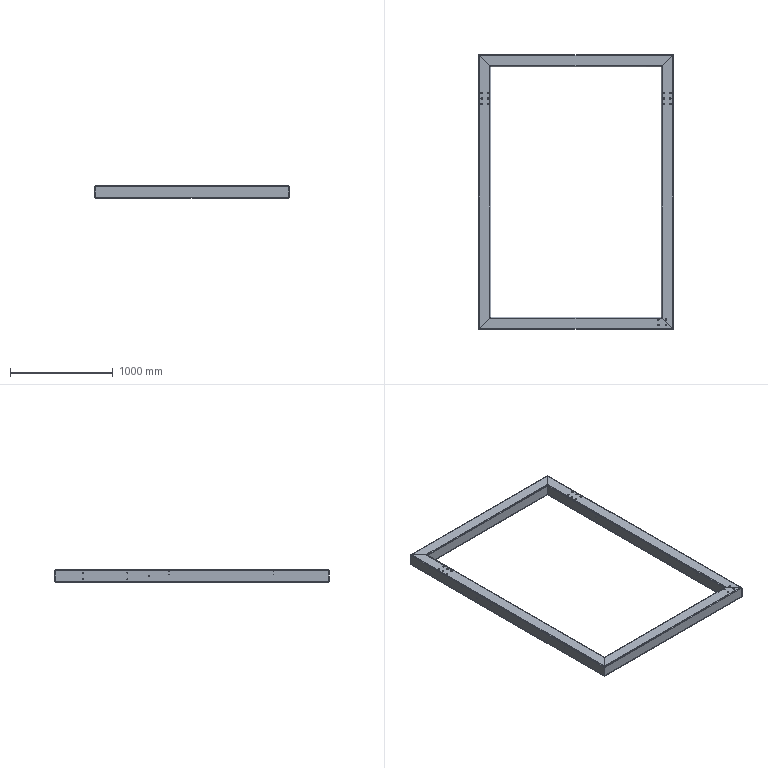Part | SolidWorks | features ICE 8, HoleWzd 6, 3DProfileFeature 1, WeldMemberFeat 1, WeldmentFeature 1 | 4 solids | 244 faces | box 1900 x 2680 x 120 mm | volume 15591720 mm3 | cylinder 204 | plane 40 | commonest cylinder face diameters 15 x92 5 x28 11 x24 20 x20 3 x16 12 x16